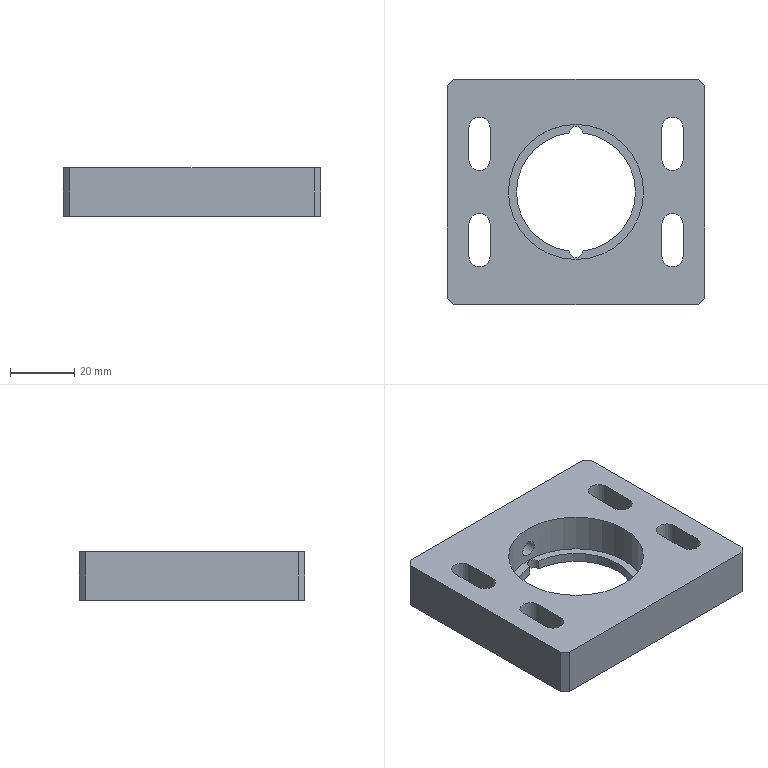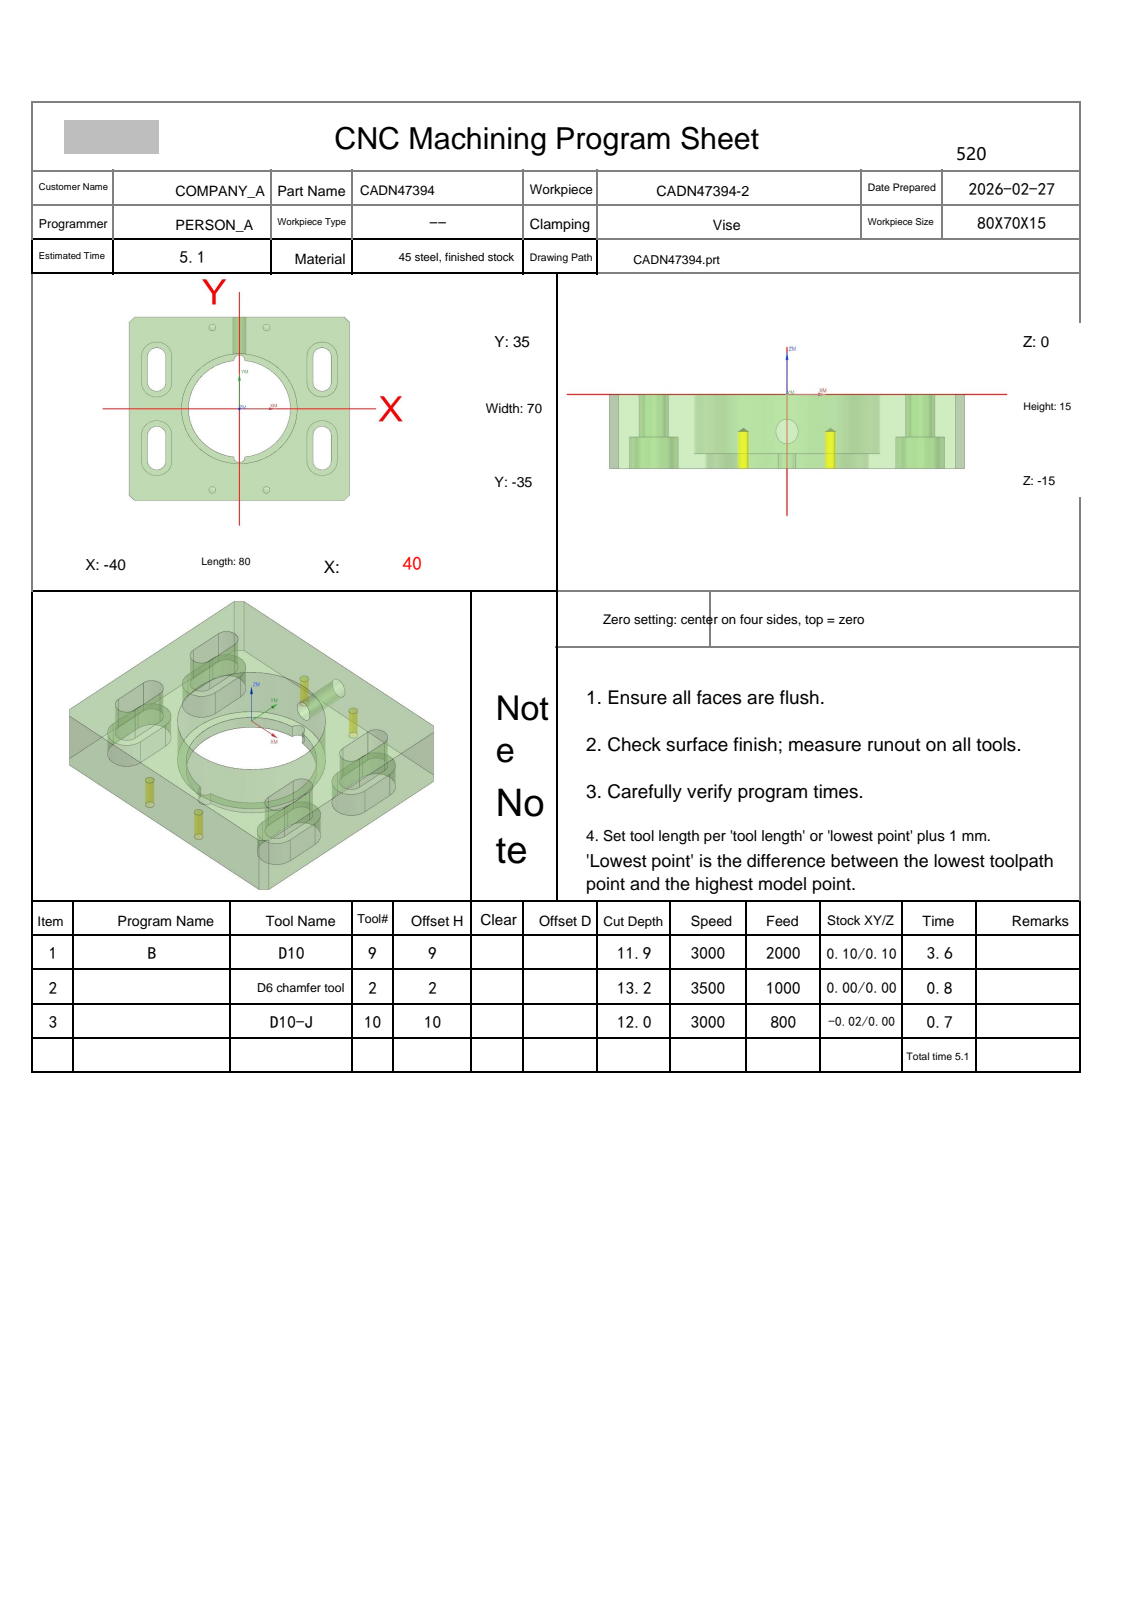NC program | NX | posted by the shop | part box 80 x 70 x 15 mm
Whole program:
%
O0001
(Machine time: 5.67 MIN)
(===Total Tool:3===)
(T9=D10     D=10.  R=0.   D-  H09 Z=-11.9 )
(T2=D6 chamfer tool   D=6.   R=0.   D-  H02 Z=-13.2 )
(T10=D10-J  D=10.  R=0.   D10 H10 Z=-12.  )
G80 G90 G17 G49 G40
G91 G28 Z0
M01
N1 T09 M06
(D10  D=10. R=0. H=09 ce=0.10 di=0.10)
G00 G90 G54 X35.242 Y44.97 M03 S3000
G43 H09 Z50.
M08
Z-.5
G01 X41.606 Y38.606 F2000.
X43.606 Y36.606
X49.97 Y30.242
G00 Z-1.
G01 X43.606 Y36.606
X41.606 Y38.606
X35.242 Y44.97
G00 Z-1.5
G01 X41.606 Y38.606
X43.606 Y36.606
X49.97 Y30.242
G00 Z-2.
G01 X43.606 Y36.606
X41.606 Y38.606
X35.242 Y44.97
G00 Z-2.5
G01 X41.606 Y38.606
X43.606 Y36.606
X49.97 Y30.242
G00 Z-3.
G01 X43.606 Y36.606
X41.606 Y38.606
X35.242 Y44.97
G00 Z-3.5
G01 X41.606 Y38.606
X43.606 Y36.606
X49.97 Y30.242
G00 Z-4.
G01 X43.606 Y36.606
X41.606 Y38.606
X35.242 Y44.97
G00 Z-4.5
G01 X41.606 Y38.606
X43.606 Y36.606
X49.97 Y30.242
G00 Z-5.
G01 X43.606 Y36.606
X41.606 Y38.606
X35.242 Y44.97
G00 Z-5.5
G01 X41.606 Y38.606
X43.606 Y36.606
X49.97 Y30.242
G00 Z-6.
G01 X43.606 Y36.606
X41.606 Y38.606
X35.242 Y44.97
G00 Z-6.5
G01 X41.606 Y38.606
X43.606 Y36.606
X49.97 Y30.242
G00 Z-7.
G01 X43.606 Y36.606
X41.606 Y38.606
X35.242 Y44.97
G00 Z-7.5
G01 X41.606 Y38.606
X43.606 Y36.606
X49.97 Y30.242
G00 Z-7.9
G01 X43.606 Y36.606
X41.606 Y38.606
X35.242 Y44.97
G00 Z50.
X49.97 Y-30.242
Z-.5
G01 X43.606 Y-36.606
X41.606 Y-38.606
X35.242 Y-44.97
G00 Z-1.
G01 X41.606 Y-38.606
X43.606 Y-36.606
X49.97 Y-30.242
G00 Z-1.5
G01 X43.606 Y-36.606
X41.606 Y-38.606
X35.242 Y-44.97
G00 Z-2.
G01 X41.606 Y-38.606
X43.606 Y-36.606
X49.97 Y-30.242
G00 Z-2.5
G01 X43.606 Y-36.606
X41.606 Y-38.606
X35.242 Y-44.97
G00 Z-3.
G01 X41.606 Y-38.606
X43.606 Y-36.606
X49.97 Y-30.242
G00 Z-3.5
G01 X43.606 Y-36.606
X41.606 Y-38.606
X35.242 Y-44.97
G00 Z-4.
G01 X41.606 Y-38.606
X43.606 Y-36.606
X49.97 Y-30.242
G00 Z-4.5
G01 X43.606 Y-36.606
X41.606 Y-38.606
X35.242 Y-44.97
G00 Z-5.
G01 X41.606 Y-38.606
X43.606 Y-36.606
X49.97 Y-30.242
G00 Z-5.5
G01 X43.606 Y-36.606
X41.606 Y-38.606
X35.242 Y-44.97
G00 Z-6.
G01 X41.606 Y-38.606
X43.606 Y-36.606
X49.97 Y-30.242
G00 Z-6.5
G01 X43.606 Y-36.606
X41.606 Y-38.606
X35.242 Y-44.97
G00 Z-7.
G01 X41.606 Y-38.606
X43.606 Y-36.606
X49.97 Y-30.242
G00 Z-7.5
G01 X43.606 Y-36.606
X41.606 Y-38.606
X35.242 Y-44.97
G00 Z-7.9
G01 X41.606 Y-38.606
X43.606 Y-36.606
X49.97 Y-30.242
G00 Z50.
X-35.242 Y-44.97
Z-.5
G01 X-41.606 Y-38.606
X-43.606 Y-36.606
X-49.97 Y-30.242
G00 Z-1.
G01 X-43.606 Y-36.606
X-41.606 Y-38.606
X-35.242 Y-44.97
G00 Z-1.5
G01 X-41.606 Y-38.606
X-43.606 Y-36.606
X-49.97 Y-30.242
G00 Z-2.
G01 X-43.606 Y-36.606
X-41.606 Y-38.606
X-35.242 Y-44.97
G00 Z-2.5
G01 X-41.606 Y-38.606
X-43.606 Y-36.606
X-49.97 Y-30.242
G00 Z-3.
G01 X-43.606 Y-36.606
X-41.606 Y-38.606
X-35.242 Y-44.97
G00 Z-3.5
G01 X-41.606 Y-38.606
X-43.606 Y-36.606
X-49.97 Y-30.242
G00 Z-4.
G01 X-43.606 Y-36.606
X-41.606 Y-38.606
X-35.242 Y-44.97
G00 Z-4.5
G01 X-41.606 Y-38.606
X-43.606 Y-36.606
X-49.97 Y-30.242
G00 Z-5.
G01 X-43.606 Y-36.606
X-41.606 Y-38.606
X-35.242 Y-44.97
G00 Z-5.5
G01 X-41.606 Y-38.606
X-43.606 Y-36.606
X-49.97 Y-30.242
G00 Z-6.
G01 X-43.606 Y-36.606
X-41.606 Y-38.606
X-35.242 Y-44.97
G00 Z-6.5
G01 X-41.606 Y-38.606
X-43.606 Y-36.606
X-49.97 Y-30.242
G00 Z-7.
G01 X-43.606 Y-36.606
X-41.606 Y-38.606
X-35.242 Y-44.97
G00 Z-7.5
G01 X-41.606 Y-38.606
X-43.606 Y-36.606
X-49.97 Y-30.242
G00 Z-7.9
G01 X-43.606 Y-36.606
X-41.606 Y-38.606
X-35.242 Y-44.97
G00 Z50.
X-49.97 Y30.242
Z-.5
G01 X-43.606 Y36.606
X-41.606 Y38.606
X-35.242 Y44.97
G00 Z-1.
G01 X-41.606 Y38.606
X-43.606 Y36.606
X-49.97 Y30.242
G00 Z-1.5
G01 X-43.606 Y36.606
X-41.606 Y38.606
X-35.242 Y44.97
G00 Z-2.
G01 X-41.606 Y38.606
X-43.606 Y36.606
X-49.97 Y30.242
G00 Z-2.5
G01 X-43.606 Y36.606
X-41.606 Y38.606
X-35.242 Y44.97
G00 Z-3.
G01 X-41.606 Y38.606
X-43.606 Y36.606
X-49.97 Y30.242
G00 Z-3.5
G01 X-43.606 Y36.606
X-41.606 Y38.606
X-35.242 Y44.97
G00 Z-4.
G01 X-41.606 Y38.606
X-43.606 Y36.606
X-49.97 Y30.242
G00 Z-4.5
G01 X-43.606 Y36.606
X-41.606 Y38.606
X-35.242 Y44.97
G00 Z-5.
G01 X-41.606 Y38.606
X-43.606 Y36.606
X-49.97 Y30.242
G00 Z-5.5
G01 X-43.606 Y36.606
X-41.606 Y38.606
X-35.242 Y44.97
G00 Z-6.
G01 X-41.606 Y38.606
X-43.606 Y36.606
X-49.97 Y30.242
G00 Z-6.5
G01 X-43.606 Y36.606
X-41.606 Y38.606
X-35.242 Y44.97
G00 Z-7.
G01 X-41.606 Y38.606
X-43.606 Y36.606
X-49.97 Y30.242
G00 Z-7.5
G01 X-43.606 Y36.606
X-41.606 Y38.606
X-35.242 Y44.97
G00 Z-7.9
G01 X-41.606 Y38.606
X-43.606 Y36.606
X-49.97 Y30.242
G00 Z50.
G00 G90 X-6.172 Y-1.54 M03 S3000
Z10.1
Z1.5
G02 X-6.172 Y-1.54 Z.018 I-4.228 J1.54 F2000.
X-14.082 Y-2.587 Z-.496 I-4.228 J1.54
G01 X-15.9 Y0.0
G02 X0.0 Y15.9 I15.9 J0.0
X15.9 Y0.0 I0.0 J-15.9
X0.0 Y-15.9 I-15.9 J0.0
X-15.9 Y0.0 I0.0 J15.9
X-15.12 Y4.918 I15.9 J0.0
X-14.169 Y5.609 I.951 J-.309
G01 X-14.078 Y5.605
X-7.936 Y5.043
X-7.845 Y5.039
G03 X-7.053 Y5.429 I0.0 J1.
G02 X0.0 Y8.9 I7.053 J-5.429
X8.9 Y0.0 I0.0 J-8.9
X0.0 Y-8.9 I-8.9 J0.0
X-8.879 Y-.609 I0.0 J8.9
G01 X-8.881 Y-.541
G02 X-8.052 Y.444 I1. J0.0
G01 X-1.012 Y1.663
G03 X-.775 Y1.735 I-.171 J.985
G02 X0.0 Y1.9 I.775 J-1.735
X1.9 Y0.0 I0.0 J-1.9
X0.0 Y-1.9 I-1.9 J0.0
X-1.9 Y0.0 I0.0 J1.9
X-1.807 Y.588 I1.9 J0.0
X-1.592 Y1.037 I1.807 J-.588
G03 X-.456 Y4.86 I-5.864 J3.822
X-3.634 Y10.724 I-7. J0.0
G01 Z.704
G00 Z3.
G01 X-6.172 Y-1.54 F6000.
G00 Z1.004
G02 X-6.172 Y-1.54 Z-.478 I-4.228 J1.54 F2000.
X-14.082 Y-2.587 Z-.992 I-4.228 J1.54
G01 X-15.9 Y0.0
G02 X0.0 Y15.9 I15.9 J0.0
X15.9 Y0.0 I0.0 J-15.9
X0.0 Y-15.9 I-15.9 J0.0
X-15.9 Y0.0 I0.0 J15.9
X-15.12 Y4.918 I15.9 J0.0
X-14.169 Y5.609 I.951 J-.309
G01 X-14.078 Y5.605
X-7.936 Y5.043
X-7.845 Y5.039
G03 X-7.053 Y5.429 I0.0 J1.
G02 X0.0 Y8.9 I7.053 J-5.429
X8.9 Y0.0 I0.0 J-8.9
X0.0 Y-8.9 I-8.9 J0.0
X-8.88 Y-.599 I0.0 J8.9
G01 X-8.882 Y-.532
G02 X-8.063 Y.451 I1. J0.0
G01 X-.331 Y1.871
X-.318 Y1.873
G02 X0.0 Y1.9 I.318 J-1.873
X1.9 Y0.0 I0.0 J-1.9
X0.0 Y-1.9 I-1.9 J0.0
X-1.9 Y0.0 I0.0 J1.9
X-1.807 Y.588 I1.9 J0.0
X-1.592 Y1.037 I1.807 J-.588
G03 X-.456 Y4.86 I-5.864 J3.822
X-3.634 Y10.724 I-7. J0.0
G01 Z.208
G00 Z2.504
G01 X-6.172 Y-1.54 F6000.
G00 Z.508
G02 X-6.172 Y-1.54 Z-.973 I-4.228 J1.54 F2000.
X-14.082 Y-2.587 Z-1.488 I-4.228 J1.54
G01 X-15.9 Y0.0
G02 X0.0 Y15.9 I15.9 J0.0
X15.9 Y0.0 I0.0 J-15.9
X0.0 Y-15.9 I-15.9 J0.0
X-15.9 Y0.0 I0.0 J15.9
X-15.12 Y4.918 I15.9 J0.0
X-14.169 Y5.609 I.951 J-.309
G01 X-14.078 Y5.605
X-7.936 Y5.043
X-7.845 Y5.039
G03 X-7.053 Y5.429 I0.0 J1.
G02 X0.0 Y8.9 I7.053 J-5.429
X8.9 Y0.0 I0.0 J-8.9
X0.0 Y-8.9 I-8.9 J0.0
X-8.88 Y-.599 I0.0 J8.9
G01 X-8.882 Y-.532
G02 X-8.063 Y.451 I1. J0.0
G01 X-.368 Y1.864
X-.36 Y1.866
G02 X0.0 Y1.9 I.36 J-1.866
X1.9 Y0.0 I0.0 J-1.9
X0.0 Y-1.9 I-1.9 J0.0
X-1.9 Y0.0 I0.0 J1.9
X-1.807 Y.588 I1.9 J0.0
X-1.592 Y1.037 I1.807 J-.588
G03 X-.456 Y4.86 I-5.864 J3.822
X-3.634 Y10.724 I-7. J0.0
G01 Z-.288
G00 Z2.008
G01 X-6.172 Y-1.54 F6000.
G00 Z.013
G02 X-6.172 Y-1.54 Z-1.469 I-4.228 J1.54 F2000.
X-14.082 Y-2.587 Z-1.983 I-4.228 J1.54
G01 X-15.9 Y0.0
G02 X0.0 Y15.9 I15.9 J0.0
X15.9 Y0.0 I0.0 J-15.9
X0.0 Y-15.9 I-15.9 J0.0
X-15.9 Y0.0 I0.0 J15.9
X-15.12 Y4.918 I15.9 J0.0
X-14.169 Y5.609 I.951 J-.309
G01 X-14.078 Y5.605
X-7.936 Y5.043
X-7.845 Y5.039
G03 X-7.053 Y5.429 I0.0 J1.
G02 X0.0 Y8.9 I7.053 J-5.429
X8.9 Y0.0 I0.0 J-8.9
X0.0 Y-8.9 I-8.9 J0.0
X-8.878 Y-.628 I0.0 J8.9
G01 X-8.88 Y-.565
G02 X-8.017 Y.334 I.9 J0.0
G01 X-2.402 Y.563
G03 X-1.601 Y1.024 I-.041 J.999
G02 X0.0 Y1.9 I1.601 J-1.024
X1.9 Y0.0 I0.0 J-1.9
X0.0 Y-1.9 I-1.9 J0.0
X-1.9 Y0.0 I0.0 J1.9
X-1.807 Y.588 I1.9 J0.0
X-1.592 Y1.037 I1.807 J-.588
G03 X-.456 Y4.86 I-5.864 J3.822
X-3.634 Y10.724 I-7. J0.0
G01 Z-.783
G00 Z1.513
G01 X-6.172 Y-1.54 F6000.
G00 Z-.483
G02 X-6.172 Y-1.54 Z-1.965 I-4.228 J1.54 F2000.
X-14.082 Y-2.587 Z-2.479 I-4.228 J1.54
G01 X-15.9 Y0.0
G02 X0.0 Y15.9 I15.9 J0.0
X15.9 Y0.0 I0.0 J-15.9
X0.0 Y-15.9 I-15.9 J0.0
X-15.9 Y0.0 I0.0 J15.9
X-15.12 Y4.918 I15.9 J0.0
X-14.169 Y5.609 I.951 J-.309
G01 X-14.078 Y5.605
X-7.936 Y5.043
X-7.845 Y5.039
G03 X-7.053 Y5.429 I0.0 J1.
G02 X0.0 Y8.9 I7.053 J-5.429
X8.9 Y0.0 I0.0 J-8.9
X0.0 Y-8.9 I-8.9 J0.0
X-8.878 Y-.628 I0.0 J8.9
G01 X-8.88 Y-.565
G02 X-8.017 Y.334 I.9 J0.0
G01 X-2.402 Y.563
G03 X-1.601 Y1.024 I-.041 J.999
G02 X0.0 Y1.9 I1.601 J-1.024
X1.9 Y0.0 I0.0 J-1.9
X0.0 Y-1.9 I-1.9 J0.0
X-1.9 Y0.0 I0.0 J1.9
X-1.807 Y.588 I1.9 J0.0
X-1.592 Y1.037 I1.807 J-.588
G03 X-.456 Y4.86 I-5.864 J3.822
X-3.634 Y10.724 I-7. J0.0
G01 Z-1.279
G00 Z1.017
G01 X-6.172 Y-1.54 F6000.
G00 Z-.979
G02 X-6.172 Y-1.54 Z-2.461 I-4.228 J1.54 F2000.
X-14.082 Y-2.587 Z-2.975 I-4.228 J1.54
G01 X-15.9 Y0.0
G02 X0.0 Y15.9 I15.9 J0.0
X15.9 Y0.0 I0.0 J-15.9
X0.0 Y-15.9 I-15.9 J0.0
X-15.9 Y0.0 I0.0 J15.9
X-15.12 Y4.918 I15.9 J0.0
X-14.169 Y5.609 I.951 J-.309
G01 X-14.078 Y5.605
X-7.936 Y5.043
X-7.845 Y5.039
G03 X-7.053 Y5.429 I0.0 J1.
G02 X0.0 Y8.9 I7.053 J-5.429
X8.9 Y0.0 I0.0 J-8.9
X0.0 Y-8.9 I-8.9 J0.0
X-8.878 Y-.628 I0.0 J8.9
G01 X-8.88 Y-.565
G02 X-8.017 Y.334 I.9 J0.0
G01 X-2.402 Y.563
G03 X-1.601 Y1.024 I-.041 J.999
G02 X0.0 Y1.9 I1.601 J-1.024
X1.9 Y0.0 I0.0 J-1.9
X0.0 Y-1.9 I-1.9 J0.0
X-1.9 Y0.0 I0.0 J1.9
X-1.807 Y.588 I1.9 J0.0
X-1.592 Y1.037 I1.807 J-.588
G03 X-.456 Y4.86 I-5.864 J3.822
X-3.634 Y10.724 I-7. J0.0
G01 Z-1.775
G00 Z.521
G01 X-6.172 Y-1.54 F6000.
G00 Z-1.475
G02 X-6.172 Y-1.54 Z-2.957 I-4.228 J1.54 F2000.
X-14.082 Y-2.587 Z-3.471 I-4.228 J1.54
G01 X-15.9 Y0.0
G02 X0.0 Y15.9 I15.9 J0.0
X15.9 Y0.0 I0.0 J-15.9
X0.0 Y-15.9 I-15.9 J0.0
X-15.9 Y0.0 I0.0 J15.9
X-15.12 Y4.918 I15.9 J0.0
X-14.169 Y5.609 I.951 J-.309
G01 X-14.078 Y5.605
X-7.936 Y5.043
X-7.845 Y5.039
G03 X-7.053 Y5.429 I0.0 J1.
G02 X0.0 Y8.9 I7.053 J-5.429
X8.9 Y0.0 I0.0 J-8.9
X0.0 Y-8.9 I-8.9 J0.0
X-8.878 Y-.628 I0.0 J8.9
G01 X-8.88 Y-.565
G02 X-8.017 Y.334 I.9 J0.0
G01 X-2.402 Y.563
G03 X-1.601 Y1.024 I-.041 J.999
G02 X0.0 Y1.9 I1.601 J-1.024
X1.9 Y0.0 I0.0 J-1.9
X0.0 Y-1.9 I-1.9 J0.0
X-1.9 Y0.0 I0.0 J1.9
X-1.807 Y.588 I1.9 J0.0
X-1.592 Y1.037 I1.807 J-.588
G03 X-.456 Y4.86 I-5.864 J3.822
X-3.634 Y10.724 I-7. J0.0
G01 Z-2.271
G00 Z.025
G01 X-6.172 Y-1.54 F6000.
G00 Z-1.971
G02 X-6.172 Y-1.54 Z-3.453 I-4.228 J1.54 F2000.
X-14.082 Y-2.587 Z-3.967 I-4.228 J1.54
G01 X-15.9 Y0.0
G02 X0.0 Y15.9 I15.9 J0.0
X15.9 Y0.0 I0.0 J-15.9
X0.0 Y-15.9 I-15.9 J0.0
X-15.9 Y0.0 I0.0 J15.9
X-15.12 Y4.918 I15.9 J0.0
X-14.169 Y5.609 I.951 J-.309
G01 X-14.078 Y5.605
X-7.936 Y5.043
X-7.845 Y5.039
G03 X-7.053 Y5.429 I0.0 J1.
G02 X0.0 Y8.9 I7.053 J-5.429
X8.9 Y0.0 I0.0 J-8.9
X0.0 Y-8.9 I-8.9 J0.0
X-8.878 Y-.628 I0.0 J8.9
G01 X-8.88 Y-.565
G02 X-8.017 Y.334 I.9 J0.0
G01 X-2.402 Y.563
G03 X-1.601 Y1.024 I-.041 J.999
G02 X0.0 Y1.9 I1.601 J-1.024
X1.9 Y0.0 I0.0 J-1.9
X0.0 Y-1.9 I-1.9 J0.0
X-1.9 Y0.0 I0.0 J1.9
X-1.807 Y.588 I1.9 J0.0
X-1.592 Y1.037 I1.807 J-.588
G03 X-.456 Y4.86 I-5.864 J3.822
X-3.634 Y10.724 I-7. J0.0
G01 Z-2.767
G00 Z-.471
G01 X-6.172 Y-1.54 F6000.
G00 Z-2.467
G02 X-6.172 Y-1.54 Z-3.948 I-4.228 J1.54 F2000.
X-14.082 Y-2.587 Z-4.463 I-4.228 J1.54
G01 X-15.9 Y0.0
G02 X0.0 Y15.9 I15.9 J0.0
X15.9 Y0.0 I0.0 J-15.9
X0.0 Y-15.9 I-15.9 J0.0
X-15.9 Y0.0 I0.0 J15.9
X-15.12 Y4.918 I15.9 J0.0
X-14.169 Y5.609 I.951 J-.309
G01 X-14.078 Y5.605
X-7.936 Y5.043
X-7.845 Y5.039
G03 X-7.053 Y5.429 I0.0 J1.
G02 X0.0 Y8.9 I7.053 J-5.429
X8.9 Y0.0 I0.0 J-8.9
X0.0 Y-8.9 I-8.9 J0.0
X-8.878 Y-.628 I0.0 J8.9
G01 X-8.88 Y-.565
G02 X-8.017 Y.334 I.9 J0.0
G01 X-2.402 Y.563
G03 X-1.601 Y1.024 I-.041 J.999
G02 X0.0 Y1.9 I1.601 J-1.024
X1.9 Y0.0 I0.0 J-1.9
X0.0 Y-1.9 I-1.9 J0.0
X-1.9 Y0.0 I0.0 J1.9
X-1.807 Y.588 I1.9 J0.0
X-1.592 Y1.037 I1.807 J-.588
G03 X-.456 Y4.86 I-5.864 J3.822
X-3.634 Y10.724 I-7. J0.0
G01 Z-3.263
G00 Z-.967
G01 X-6.172 Y-1.54 F6000.
G00 Z-2.963
G02 X-6.172 Y-1.54 Z-4.444 I-4.228 J1.54 F2000.
X-14.082 Y-2.587 Z-4.958 I-4.228 J1.54
G01 X-15.9 Y0.0
G02 X0.0 Y15.9 I15.9 J0.0
X15.9 Y0.0 I0.0 J-15.9
X0.0 Y-15.9 I-15.9 J0.0
X-15.9 Y0.0 I0.0 J15.9
X-15.12 Y4.918 I15.9 J0.0
X-14.169 Y5.609 I.951 J-.309
G01 X-14.078 Y5.605
X-7.936 Y5.043
X-7.845 Y5.039
G03 X-7.053 Y5.429 I0.0 J1.
G02 X0.0 Y8.9 I7.053 J-5.429
X8.9 Y0.0 I0.0 J-8.9
X0.0 Y-8.9 I-8.9 J0.0
X-8.878 Y-.628 I0.0 J8.9
G01 X-8.88 Y-.565
G02 X-8.017 Y.334 I.9 J0.0
G01 X-2.402 Y.563
G03 X-1.601 Y1.024 I-.041 J.999
G02 X0.0 Y1.9 I1.601 J-1.024
X1.9 Y0.0 I0.0 J-1.9
X0.0 Y-1.9 I-1.9 J0.0
X-1.9 Y0.0 I0.0 J1.9
X-1.807 Y.588 I1.9 J0.0
X-1.592 Y1.037 I1.807 J-.588
G03 X-.456 Y4.86 I-5.864 J3.822
X-3.634 Y10.724 I-7. J0.0
G01 Z-3.758
G00 Z-1.463
G01 X-6.172 Y-1.54 F6000.
G00 Z-3.458
G02 X-6.172 Y-1.54 Z-4.94 I-4.228 J1.54 F2000.
X-14.082 Y-2.587 Z-5.454 I-4.228 J1.54
G01 X-15.9 Y0.0
G02 X0.0 Y15.9 I15.9 J0.0
X15.9 Y0.0 I0.0 J-15.9
X0.0 Y-15.9 I-15.9 J0.0
X-15.9 Y0.0 I0.0 J15.9
X-15.12 Y4.918 I15.9 J0.0
X-14.169 Y5.609 I.951 J-.309
G01 X-14.078 Y5.605
X-7.936 Y5.043
X-7.845 Y5.039
G03 X-7.053 Y5.429 I0.0 J1.
G02 X0.0 Y8.9 I7.053 J-5.429
X8.9 Y0.0 I0.0 J-8.9
X0.0 Y-8.9 I-8.9 J0.0
X-8.878 Y-.628 I0.0 J8.9
G01 X-8.88 Y-.565
G02 X-8.017 Y.334 I.9 J0.0
G01 X-2.402 Y.563
G03 X-1.601 Y1.024 I-.041 J.999
G02 X0.0 Y1.9 I1.601 J-1.024
X1.9 Y0.0 I0.0 J-1.9
X0.0 Y-1.9 I-1.9 J0.0
X-1.9 Y0.0 I0.0 J1.9
X-1.807 Y.588 I1.9 J0.0
X-1.592 Y1.037 I1.807 J-.588
G03 X-.456 Y4.86 I-5.864 J3.822
X-3.634 Y10.724 I-7. J0.0
G01 Z-4.254
G00 Z-1.958
G01 X-6.172 Y-1.54 F6000.
G00 Z-3.954
G02 X-6.172 Y-1.54 Z-5.436 I-4.228 J1.54 F2000.
X-14.082 Y-2.587 Z-5.95 I-4.228 J1.54
G01 X-15.9 Y0.0
G02 X0.0 Y15.9 I15.9 J0.0
X15.9 Y0.0 I0.0 J-15.9
X0.0 Y-15.9 I-15.9 J0.0
X-15.9 Y0.0 I0.0 J15.9
X-15.12 Y4.918 I15.9 J0.0
X-14.169 Y5.609 I.951 J-.309
G01 X-14.078 Y5.605
X-7.936 Y5.043
X-7.845 Y5.039
G03 X-7.053 Y5.429 I0.0 J1.
G02 X0.0 Y8.9 I7.053 J-5.429
X8.9 Y0.0 I0.0 J-8.9
X0.0 Y-8.9 I-8.9 J0.0
X-8.878 Y-.628 I0.0 J8.9
G01 X-8.88 Y-.565
G02 X-8.017 Y.334 I.9 J0.0
G01 X-2.402 Y.563
G03 X-1.601 Y1.024 I-.041 J.999
G02 X0.0 Y1.9 I1.601 J-1.024
X1.9 Y0.0 I0.0 J-1.9
X0.0 Y-1.9 I-1.9 J0.0
X-1.9 Y0.0 I0.0 J1.9
X-1.807 Y.588 I1.9 J0.0
X-1.592 Y1.037 I1.807 J-.588
G03 X-.456 Y4.86 I-5.864 J3.822
X-3.634 Y10.724 I-7. J0.0
G01 Z-4.75
G00 Z-2.454
G01 X-6.172 Y-1.54 F6000.
G00 Z-4.45
G02 X-6.172 Y-1.54 Z-5.932 I-4.228 J1.54 F2000.
X-14.082 Y-2.587 Z-6.446 I-4.228 J1.54
G01 X-15.9 Y0.0
G02 X0.0 Y15.9 I15.9 J0.0
X15.9 Y0.0 I0.0 J-15.9
X0.0 Y-15.9 I-15.9 J0.0
X-15.9 Y0.0 I0.0 J15.9
X-15.12 Y4.918 I15.9 J0.0
X-14.169 Y5.609 I.951 J-.309
G01 X-14.078 Y5.605
X-7.936 Y5.043
X-7.845 Y5.039
G03 X-7.053 Y5.429 I0.0 J1.
G02 X0.0 Y8.9 I7.053 J-5.429
X8.9 Y0.0 I0.0 J-8.9
X0.0 Y-8.9 I-8.9 J0.0
X-8.878 Y-.628 I0.0 J8.9
G01 X-8.88 Y-.565
G02 X-8.017 Y.334 I.9 J0.0
G01 X-2.402 Y.563
G03 X-1.601 Y1.024 I-.041 J.999
G02 X0.0 Y1.9 I1.601 J-1.024
X1.9 Y0.0 I0.0 J-1.9
X0.0 Y-1.9 I-1.9 J0.0
X-1.9 Y0.0 I0.0 J1.9
X-1.807 Y.588 I1.9 J0.0
X-1.592 Y1.037 I1.807 J-.588
G03 X-.456 Y4.86 I-5.864 J3.822
X-3.634 Y10.724 I-7. J0.0
G01 Z-5.246
G00 Z-2.95
G01 X-6.172 Y-1.54 F6000.
G00 Z-4.946
G02 X-6.172 Y-1.54 Z-6.428 I-4.228 J1.54 F2000.
X-14.082 Y-2.587 Z-6.942 I-4.228 J1.54
G01 X-15.9 Y0.0
G02 X0.0 Y15.9 I15.9 J0.0
X15.9 Y0.0 I0.0 J-15.9
X0.0 Y-15.9 I-15.9 J0.0
X-15.9 Y0.0 I0.0 J15.9
X-15.12 Y4.918 I15.9 J0.0
X-14.169 Y5.609 I.951 J-.309
G01 X-14.078 Y5.605
X-7.936 Y5.043
X-7.845 Y5.039
G03 X-7.053 Y5.429 I0.0 J1.
G02 X0.0 Y8.9 I7.053 J-5.429
X8.9 Y0.0 I0.0 J-8.9
X0.0 Y-8.9 I-8.9 J0.0
X-8.878 Y-.628 I0.0 J8.9
G01 X-8.88 Y-.565
G02 X-8.017 Y.334 I.9 J0.0
G01 X-2.402 Y.563
G03 X-1.601 Y1.024 I-.041 J.999
G02 X0.0 Y1.9 I1.601 J-1.024
X1.9 Y0.0 I0.0 J-1.9
X0.0 Y-1.9 I-1.9 J0.0
X-1.9 Y0.0 I0.0 J1.9
X-1.807 Y.588 I1.9 J0.0
X-1.592 Y1.037 I1.807 J-.588
G03 X-.456 Y4.86 I-5.864 J3.822
X-3.634 Y10.724 I-7. J0.0
G01 Z-5.742
G00 Z-3.446
G01 X-6.172 Y-1.54 F6000.
G00 Z-5.442
G02 X-6.172 Y-1.54 Z-6.923 I-4.228 J1.54 F2000.
X-14.082 Y-2.587 Z-7.438 I-4.228 J1.54
G01 X-15.9 Y0.0
G02 X0.0 Y15.9 I15.9 J0.0
X15.9 Y0.0 I0.0 J-15.9
X0.0 Y-15.9 I-15.9 J0.0
X-15.9 Y0.0 I0.0 J15.9
X-15.12 Y4.918 I15.9 J0.0
X-14.169 Y5.609 I.951 J-.309
G01 X-14.078 Y5.605
X-7.936 Y5.043
X-7.845 Y5.039
G03 X-7.053 Y5.429 I0.0 J1.
G02 X0.0 Y8.9 I7.053 J-5.429
X8.9 Y0.0 I0.0 J-8.9
X0.0 Y-8.9 I-8.9 J0.0
X-8.878 Y-.628 I0.0 J8.9
G01 X-8.88 Y-.565
G02 X-8.017 Y.334 I.9 J0.0
G01 X-2.402 Y.563
G03 X-1.601 Y1.024 I-.041 J.999
G02 X0.0 Y1.9 I1.601 J-1.024
X1.9 Y0.0 I0.0 J-1.9
X0.0 Y-1.9 I-1.9 J0.0
X-1.9 Y0.0 I0.0 J1.9
X-1.807 Y.588 I1.9 J0.0
X-1.592 Y1.037 I1.807 J-.588
G03 X-.456 Y4.86 I-5.864 J3.822
X-3.634 Y10.724 I-7. J0.0
G01 Z-6.238
G00 Z-3.942
G01 X-6.172 Y-1.54 F6000.
G00 Z-5.938
G02 X-6.172 Y-1.54 Z-7.419 I-4.228 J1.54 F2000.
X-14.082 Y-2.587 Z-7.933 I-4.228 J1.54
G01 X-15.9 Y0.0
G02 X0.0 Y15.9 I15.9 J0.0
X15.9 Y0.0 I0.0 J-15.9
X0.0 Y-15.9 I-15.9 J0.0
X-15.9 Y0.0 I0.0 J15.9
X-15.12 Y4.918 I15.9 J0.0
X-14.169 Y5.609 I.951 J-.309
G01 X-14.078 Y5.605
X-7.936 Y5.043
X-7.845 Y5.039
G03 X-7.053 Y5.429 I0.0 J1.
G02 X0.0 Y8.9 I7.053 J-5.429
X8.9 Y0.0 I0.0 J-8.9
X0.0 Y-8.9 I-8.9 J0.0
X-8.878 Y-.628 I0.0 J8.9
G01 X-8.88 Y-.565
G02 X-8.017 Y.334 I.9 J0.0
G01 X-2.402 Y.563
G03 X-1.601 Y1.024 I-.041 J.999
G02 X0.0 Y1.9 I1.601 J-1.024
X1.9 Y0.0 I0.0 J-1.9
X0.0 Y-1.9 I-1.9 J0.0
X-1.9 Y0.0 I0.0 J1.9
X-1.807 Y.588 I1.9 J0.0
X-1.592 Y1.037 I1.807 J-.588
G03 X-.456 Y4.86 I-5.864 J3.822
X-3.634 Y10.724 I-7. J0.0
G01 Z-6.733
G00 Z-4.438
G01 X-6.172 Y-1.54 F6000.
G00 Z-6.433
G02 X-6.172 Y-1.54 Z-7.915 I-4.228 J1.54 F2000.
X-14.082 Y-2.587 Z-8.429 I-4.228 J1.54
G01 X-15.9 Y0.0
G02 X0.0 Y15.9 I15.9 J0.0
X15.9 Y0.0 I0.0 J-15.9
X0.0 Y-15.9 I-15.9 J0.0
X-15.9 Y0.0 I0.0 J15.9
X-15.12 Y4.918 I15.9 J0.0
X-14.169 Y5.609 I.951 J-.309
G01 X-14.078 Y5.605
X-7.936 Y5.043
X-7.845 Y5.039
G03 X-7.053 Y5.429 I0.0 J1.
G02 X0.0 Y8.9 I7.053 J-5.429
X8.9 Y0.0 I0.0 J-8.9
X0.0 Y-8.9 I-8.9 J0.0
X-8.878 Y-.628 I0.0 J8.9
G01 X-8.88 Y-.565
G02 X-8.017 Y.334 I.9 J0.0
G01 X-2.402 Y.563
G03 X-1.601 Y1.024 I-.041 J.999
G02 X0.0 Y1.9 I1.601 J-1.024
X1.9 Y0.0 I0.0 J-1.9
X0.0 Y-1.9 I-1.9 J0.0
X-1.9 Y0.0 I0.0 J1.9
X-1.807 Y.588 I1.9 J0.0
X-1.592 Y1.037 I1.807 J-.588
G03 X-.456 Y4.86 I-5.864 J3.822
X-3.634 Y10.724 I-7. J0.0
G01 Z-7.229
G00 Z-4.933
G01 X-6.172 Y-1.54 F6000.
G00 Z-6.929
G02 X-6.172 Y-1.54 Z-8.411 I-4.228 J1.54 F2000.
X-14.082 Y-2.587 Z-8.925 I-4.228 J1.54
G01 X-15.9 Y0.0
G02 X0.0 Y15.9 I15.9 J0.0
X15.9 Y0.0 I0.0 J-15.9
X0.0 Y-15.9 I-15.9 J0.0
X-15.9 Y0.0 I0.0 J15.9
X-15.12 Y4.918 I15.9 J0.0
X-14.169 Y5.609 I.951 J-.309
G01 X-14.078 Y5.605
X-7.936 Y5.043
X-7.845 Y5.039
G03 X-7.053 Y5.429 I0.0 J1.
G02 X0.0 Y8.9 I7.053 J-5.429
X8.9 Y0.0 I0.0 J-8.9
X0.0 Y-8.9 I-8.9 J0.0
X-8.878 Y-.628 I0.0 J8.9
G01 X-8.88 Y-.565
G02 X-8.017 Y.334 I.9 J0.0
G01 X-2.402 Y.563
G03 X-1.601 Y1.024 I-.041 J.999
G02 X0.0 Y1.9 I1.601 J-1.024
X1.9 Y0.0 I0.0 J-1.9
X0.0 Y-1.9 I-1.9 J0.0
X-1.9 Y0.0 I0.0 J1.9
X-1.807 Y.588 I1.9 J0.0
X-1.592 Y1.037 I1.807 J-.588
G03 X-.456 Y4.86 I-5.864 J3.822
X-3.634 Y10.724 I-7. J0.0
G01 Z-7.725
G00 Z-5.429
G01 X-6.172 Y-1.54 F6000.
G00 Z-7.425
G02 X-6.172 Y-1.54 Z-8.907 I-4.228 J1.54 F2000.
X-14.082 Y-2.587 Z-9.421 I-4.228 J1.54
G01 X-15.9 Y0.0
G02 X0.0 Y15.9 I15.9 J0.0
X15.9 Y0.0 I0.0 J-15.9
X0.0 Y-15.9 I-15.9 J0.0
X-15.9 Y0.0 I0.0 J15.9
X-15.12 Y4.918 I15.9 J0.0
X-14.169 Y5.609 I.951 J-.309
G01 X-14.078 Y5.605
X-7.936 Y5.043
X-7.845 Y5.039
G03 X-7.053 Y5.429 I0.0 J1.
G02 X0.0 Y8.9 I7.053 J-5.429
X8.9 Y0.0 I0.0 J-8.9
X0.0 Y-8.9 I-8.9 J0.0
X-8.878 Y-.628 I0.0 J8.9
G01 X-8.88 Y-.565
G02 X-8.017 Y.334 I.9 J0.0
G01 X-2.402 Y.563
G03 X-1.601 Y1.024 I-.041 J.999
G02 X0.0 Y1.9 I1.601 J-1.024
X1.9 Y0.0 I0.0 J-1.9
X0.0 Y-1.9 I-1.9 J0.0
X-1.9 Y0.0 I0.0 J1.9
X-1.807 Y.588 I1.9 J0.0
X-1.592 Y1.037 I1.807 J-.588
G03 X-.456 Y4.86 I-5.864 J3.822
X-3.634 Y10.724 I-7. J0.0
G01 Z-8.221
G00 Z-5.925
G01 X-6.172 Y-1.54 F6000.
G00 Z-7.921
G02 X-6.172 Y-1.54 Z-9.403 I-4.228 J1.54 F2000.
X-14.082 Y-2.587 Z-9.917 I-4.228 J1.54
G01 X-15.9 Y0.0
G02 X0.0 Y15.9 I15.9 J0.0
X15.9 Y0.0 I0.0 J-15.9
X0.0 Y-15.9 I-15.9 J0.0
X-15.9 Y0.0 I0.0 J15.9
X-15.12 Y4.918 I15.9 J0.0
X-14.169 Y5.609 I.951 J-.309
G01 X-14.078 Y5.605
X-7.936 Y5.043
X-7.845 Y5.039
G03 X-7.053 Y5.429 I0.0 J1.
G02 X0.0 Y8.9 I7.053 J-5.429
X8.9 Y0.0 I0.0 J-8.9
X0.0 Y-8.9 I-8.9 J0.0
X-8.878 Y-.628 I0.0 J8.9
G01 X-8.88 Y-.565
G02 X-8.017 Y.334 I.9 J0.0
G01 X-2.402 Y.563
G03 X-1.601 Y1.024 I-.041 J.999
G02 X0.0 Y1.9 I1.601 J-1.024
X1.9 Y0.0 I0.0 J-1.9
X0.0 Y-1.9 I-1.9 J0.0
X-1.9 Y0.0 I0.0 J1.9
X-1.807 Y.588 I1.9 J0.0
X-1.592 Y1.037 I1.807 J-.588
G03 X-.456 Y4.86 I-5.864 J3.822
X-3.634 Y10.724 I-7. J0.0
G01 Z-8.717
G00 Z-6.421
G01 X-6.172 Y-1.54 F6000.
G00 Z-8.417
G02 X-6.172 Y-1.54 Z-9.898 I-4.228 J1.54 F2000.
X-14.082 Y-2.587 Z-10.413 I-4.228 J1.54
G01 X-15.9 Y0.0
G02 X0.0 Y15.9 I15.9 J0.0
X15.9 Y0.0 I0.0 J-15.9
X0.0 Y-15.9 I-15.9 J0.0
X-15.9 Y0.0 I0.0 J15.9
X-15.12 Y4.918 I15.9 J0.0
X-14.169 Y5.609 I.951 J-.309
G01 X-14.078 Y5.605
X-7.936 Y5.043
X-7.845 Y5.039
G03 X-7.053 Y5.429 I0.0 J1.
G02 X0.0 Y8.9 I7.053 J-5.429
X8.9 Y0.0 I0.0 J-8.9
X0.0 Y-8.9 I-8.9 J0.0
X-8.878 Y-.628 I0.0 J8.9
G01 X-8.88 Y-.565
G02 X-8.017 Y.334 I.9 J0.0
G01 X-2.402 Y.563
G03 X-1.601 Y1.024 I-.041 J.999
G02 X0.0 Y1.9 I1.601 J-1.024
X1.9 Y0.0 I0.0 J-1.9
X0.0 Y-1.9 I-1.9 J0.0
X-1.9 Y0.0 I0.0 J1.9
X-1.807 Y.588 I1.9 J0.0
X-1.592 Y1.037 I1.807 J-.588
G03 X-.456 Y4.86 I-5.864 J3.822
X-3.634 Y10.724 I-7. J0.0
G01 Z-9.213
G00 Z-6.917
G01 X-6.172 Y-1.54 F6000.
G00 Z-8.913
G02 X-6.172 Y-1.54 Z-10.394 I-4.228 J1.54 F2000.
X-14.082 Y-2.587 Z-10.908 I-4.228 J1.54
G01 X-15.9 Y0.0
G02 X0.0 Y15.9 I15.9 J0.0
X15.9 Y0.0 I0.0 J-15.9
X0.0 Y-15.9 I-15.9 J0.0
X-15.9 Y0.0 I0.0 J15.9
X-15.12 Y4.918 I15.9 J0.0
X-14.169 Y5.609 I.951 J-.309
G01 X-14.078 Y5.605
X-7.936 Y5.043
X-7.845 Y5.039
G03 X-7.053 Y5.429 I0.0 J1.
G02 X0.0 Y8.9 I7.053 J-5.429
X8.9 Y0.0 I0.0 J-8.9
X0.0 Y-8.9 I-8.9 J0.0
X-8.878 Y-.628 I0.0 J8.9
G01 X-8.88 Y-.565
G02 X-8.017 Y.334 I.9 J0.0
G01 X-2.402 Y.563
G03 X-1.601 Y1.024 I-.041 J.999
G02 X0.0 Y1.9 I1.601 J-1.024
X1.9 Y0.0 I0.0 J-1.9
X0.0 Y-1.9 I-1.9 J0.0
X-1.9 Y0.0 I0.0 J1.9
X-1.807 Y.588 I1.9 J0.0
X-1.592 Y1.037 I1.807 J-.588
G03 X-.456 Y4.86 I-5.864 J3.822
X-3.634 Y10.724 I-7. J0.0
G01 Z-9.708
G00 Z-7.413
G01 X-6.172 Y-1.54 F6000.
G00 Z-9.408
G02 X-6.172 Y-1.54 Z-10.89 I-4.228 J1.54 F2000.
X-14.082 Y-2.587 Z-11.404 I-4.228 J1.54
G01 X-15.9 Y0.0
G02 X0.0 Y15.9 I15.9 J0.0
X15.9 Y0.0 I0.0 J-15.9
X0.0 Y-15.9 I-15.9 J0.0
X-15.9 Y0.0 I0.0 J15.9
X-15.12 Y4.918 I15.9 J0.0
X-14.169 Y5.609 I.951 J-.309
G01 X-14.078 Y5.605
X-7.936 Y5.043
X-7.845 Y5.039
G03 X-7.053 Y5.429 I0.0 J1.
G02 X0.0 Y8.9 I7.053 J-5.429
X8.9 Y0.0 I0.0 J-8.9
X0.0 Y-8.9 I-8.9 J0.0
X-8.878 Y-.628 I0.0 J8.9
G01 X-8.88 Y-.565
G02 X-8.017 Y.334 I.9 J0.0
G01 X-2.402 Y.563
G03 X-1.601 Y1.024 I-.041 J.999
G02 X0.0 Y1.9 I1.601 J-1.024
X1.9 Y0.0 I0.0 J-1.9
X0.0 Y-1.9 I-1.9 J0.0
X-1.9 Y0.0 I0.0 J1.9
X-1.807 Y.588 I1.9 J0.0
X-1.592 Y1.037 I1.807 J-.588
G03 X-.456 Y4.86 I-5.864 J3.822
X-3.634 Y10.724 I-7. J0.0
G01 Z-10.204
G00 Z-7.908
G01 X-6.172 Y-1.54 F6000.
G00 Z-9.904
G02 X-6.172 Y-1.54 Z-11.386 I-4.228 J1.54 F2000.
X-14.082 Y-2.587 Z-11.9 I-4.228 J1.54
G01 X-15.9 Y0.0
G02 X0.0 Y15.9 I15.9 J0.0
X15.9 Y0.0 I0.0 J-15.9
X0.0 Y-15.9 I-15.9 J0.0
X-15.9 Y0.0 I0.0 J15.9
X-15.12 Y4.918 I15.9 J0.0
X-14.169 Y5.609 I.951 J-.309
G01 X-14.078 Y5.605
X-7.936 Y5.043
X-7.845 Y5.039
G03 X-7.053 Y5.429 I0.0 J1.
G02 X0.0 Y8.9 I7.053 J-5.429
X8.9 Y0.0 I0.0 J-8.9
X0.0 Y-8.9 I-8.9 J0.0
X-8.878 Y-.628 I0.0 J8.9
G01 X-8.88 Y-.565
G02 X-8.017 Y.334 I.9 J0.0
G01 X-2.402 Y.563
G03 X-1.601 Y1.024 I-.041 J.999
G02 X0.0 Y1.9 I1.601 J-1.024
X1.9 Y0.0 I0.0 J-1.9
X0.0 Y-1.9 I-1.9 J0.0
X-1.9 Y0.0 I0.0 J1.9
X-1.807 Y.588 I1.9 J0.0
X-1.592 Y1.037 I1.807 J-.588
G03 X-.456 Y4.86 I-5.864 J3.822
X-3.634 Y10.724 I-7. J0.0
G01 Z-10.7
G00 Z10.1
G91 G28 Z0.0
M05
M09
G91 G28 Z0.0
M01
N2 T02 M06
(D6 chamfer tool  D=6. R=0. H=02 ce=0.00 di=0.00)
G00 G90 G54 X-.386 Y36.227 M03 S3500
G43 H02 Z50.
M08
Z.172
G01 Z-1.2 F1000.
G03 X-.1 Y36.027 I1.286 J1.532
G01 X-.054 Y35.997
X0.0 Y36.
X38.
X38.259 Y35.966
X38.5 Y35.866
X38.707 Y35.707
X40.707 Y33.707
X40.866 Y33.5
X40.966 Y33.259
X41. Y33.
Y-33.
X40.966 Y-33.259
X40.866 Y-33.5
X40.707 Y-33.707
X38.707 Y-35.707
X38.5 Y-35.866
X38.259 Y-35.966
X38. Y-36.
X-38.
X-38.259 Y-35.966
X-38.5 Y-35.866
X-38.707 Y-35.707
X-40.707 Y-33.707
X-40.866 Y-33.5
X-40.966 Y-33.259
X-41. Y-33.
Y33.
X-40.966 Y33.259
X-40.866 Y33.5
X-40.707 Y33.707
X-38.707 Y35.707
X-38.5 Y35.866
X-38.259 Y35.966
X-38. Y36.
X0.0
X.054 Y35.997
X.1 Y36.027
G03 X.386 Y36.227 I-1. J1.732
G01 Z.172
G00 Z10.
X-27.927 Y14.614
Z.172
G01 Z-1.2
G03 X-27.727 Y14.9 I-1.532 J1.286
G01 X-27.697 Y14.946
X-27.7 Y15.
Y20.
G03 X-30. Y22.3 I-2.3 J0.0
X-32.3 Y20. I0.0 J-2.3
G01 Y10.
G03 X-30. Y7.7 I2.3 J0.0
X-27.7 Y10. I0.0 J2.3
G01 Y15.
X-27.697 Y15.054
X-27.727 Y15.1
G03 X-27.927 Y15.386 I-1.732 J-1.
G01 Z.172
G00 Z10.
Y-15.386
Z.172
G01 Z-1.2
G03 X-27.727 Y-15.1 I-1.532 J1.286
G01 X-27.697 Y-15.054
X-27.7 Y-15.
Y-10.
G03 X-30. Y-7.7 I-2.3 J0.0
X-32.3 Y-10. I0.0 J-2.3
G01 Y-20.
G03 X-30. Y-22.3 I2.3 J0.0
X-27.7 Y-20. I0.0 J2.3
G01 Y-15.
X-27.697 Y-14.946
X-27.727 Y-14.9
G03 X-27.927 Y-14.614 I-1.732 J-1.
G01 Z.172
G00 Z10.
X-19.785 Y.392
Z.197
G01 Z-1.2
G03 X-19.976 Y.101 I1.571 J-1.238
G01 X-20.005 Y.054
X-20. Y0.0
G03 X0.0 Y-20. I20. J0.0
X20. Y0.0 I0.0 J20.
X0.0 Y20. I-20. J0.0
X-20. Y0.0 I0.0 J-20.
G01 X-20.005 Y-.054
X-19.976 Y-.101
G03 X-19.785 Y-.392 I1.762 J.946
G01 Z.197
G00 Z10.
X27.927 Y-14.614
Z.172
G01 Z-1.2
G03 X27.727 Y-14.9 I1.532 J-1.286
G01 X27.697 Y-14.946
X27.7 Y-15.
Y-20.
G03 X30. Y-22.3 I2.3 J0.0
X32.3 Y-20. I0.0 J2.3
G01 Y-10.
G03 X30. Y-7.7 I-2.3 J0.0
X27.7 Y-10. I0.0 J-2.3
G01 Y-15.
X27.697 Y-15.054
X27.727 Y-15.1
G03 X27.927 Y-15.386 I1.732 J1.
G01 Z.172
G00 Z10.
Y15.386
Z.172
G01 Z-1.2
G03 X27.727 Y15.1 I1.532 J-1.286
G01 X27.697 Y15.054
X27.7 Y15.
Y10.
G03 X30. Y7.7 I2.3 J0.0
X32.3 Y10. I0.0 J2.3
G01 Y20.
G03 X30. Y22.3 I-2.3 J0.0
X27.7 Y20. I0.0 J-2.3
G01 Y15.
X27.697 Y14.946
X27.727 Y14.9
G03 X27.927 Y14.614 I1.732 J1.
G01 Z.172
G00 Z10.
X-.89 Y17.752
Z-1.818
G01 Z-13.199
G03 X-1.236 Y17.707 I.084 J-1.998
G01 X-1.29 Y17.698
X-1.328 Y17.659
X-1.421 Y17.574
X-1.644 Y17.456
X-1.889 Y17.398
G03 X-17.5 Y0.0 I1.889 J-17.398
X-1.889 Y-17.398 I17.5 J0.0
G01 X-1.644 Y-17.456
X-1.421 Y-17.574
X-1.328 Y-17.659
X-1.29 Y-17.698
X-1.236 Y-17.707
G03 X-.89 Y-17.752 I.43 J1.953
G01 Z-1.818
G00 Z1.801
X.89
Z-1.818
G01 Z-13.199
G03 X1.236 Y-17.707 I-.084 J1.998
G01 X1.29 Y-17.698
X1.328 Y-17.659
X1.421 Y-17.574
X1.644 Y-17.456
X1.889 Y-17.398
G03 X17.5 Y0.0 I-1.889 J17.398
X1.889 Y17.398 I-17.5 J0.0
G01 X1.644 Y17.456
X1.421 Y17.574
X1.328 Y17.659
X1.29 Y17.698
X1.236 Y17.707
G03 X.89 Y17.752 I-.43 J-1.953
G01 Z-1.818
G00 Z50.
G91 G28 Z0.0
M05
M09
G91 G28 Z0.0
M01
N3 T10 M06
(D10-J  D=10. R=0. H=10 ce=0.00 di=0.00)
G00 G90 G54 X-37.293 Y-42.778 M03 S3000
G43 H10 Z50.
M08
Z-7.
G01 Z-8. F800.
X-41.536 Y-38.536
X-43.536 Y-36.536
X-47.778 Y-32.293
Z-7.
G00 Z50.
Y32.293
Z-7.
G01 Z-8.
X-43.536 Y36.536
X-41.536 Y38.536
X-37.293 Y42.778
Z-7.
G00 Z50.
X37.293
Z-7.
G01 Z-8.
X41.536 Y38.536
X43.536 Y36.536
X47.778 Y32.293
Z-7.
G00 Z50.
Y-32.293
Z-7.
G01 Z-8.
X43.536 Y-36.536
X41.536 Y-38.536
X37.293 Y-42.778
Z-7.
G00 Z50.
G00 G90 X-1.5 Y-14.242 M03 S3000
Z10.
Z-4.5
G01 Z-6. F800.
G41 D10
Y-14.52
G03 X0.0 Y-16.02 I1.5 J0.0
X16.02 Y0.0 I0.0 J16.02
X0.0 Y16.02 I-16.02 J0.0
X-16.02 Y0.0 I0.0 J-16.02
X0.0 Y-16.02 I16.02 J0.0
X.4 Y-16.015 I0.0 J16.02
X1.863 Y-14.515 I-.037 J1.5
G01 X1.862 Y-14.478
X1.86 Y-14.4
G40 X1.855 Y-14.2
Z-4.5
G00 X-1.5 Y-14.242
Z-10.5
G01 Z-12.
G41 D10
Y-14.52
G03 X0.0 Y-16.02 I1.5 J0.0
X16.02 Y0.0 I0.0 J16.02
X0.0 Y16.02 I-16.02 J0.0
X-16.02 Y0.0 I0.0 J-16.02
X0.0 Y-16.02 I16.02 J0.0
X.4 Y-16.015 I0.0 J16.02
X1.863 Y-14.515 I-.037 J1.5
G01 X1.862 Y-14.478
X1.86 Y-14.4
G40 X1.855 Y-14.2
Z-10.5
G00 Z10.
G00 G90 X-1.5 Y-14.242 M03 S3000
Z10.
Z-4.5
G01 Z-6. F800.
G41 D10
Y-14.52
G03 X0.0 Y-16.02 I1.5 J0.0
X16.02 Y0.0 I0.0 J16.02
X0.0 Y16.02 I-16.02 J0.0
X-16.02 Y0.0 I0.0 J-16.02
X0.0 Y-16.02 I16.02 J0.0
X.4 Y-16.015 I0.0 J16.02
X1.863 Y-14.515 I-.037 J1.5
G01 X1.862 Y-14.478
X1.86 Y-14.4
G40 X1.855 Y-14.2
Z-4.5
G00 X-1.5 Y-14.242
Z-10.5
G01 Z-12.
G41 D10
Y-14.52
G03 X0.0 Y-16.02 I1.5 J0.0
X16.02 Y0.0 I0.0 J16.02
X0.0 Y16.02 I-16.02 J0.0
X-16.02 Y0.0 I0.0 J-16.02
X0.0 Y-16.02 I16.02 J0.0
X.4 Y-16.015 I0.0 J16.02
X1.863 Y-14.515 I-.037 J1.5
G01 X1.862 Y-14.478
X1.86 Y-14.4
G40 X1.855 Y-14.2
Z-10.5
G00 Z10.
M05
M09
G91 G28 Z0.0
G91 G28 Y0.0
M30
%